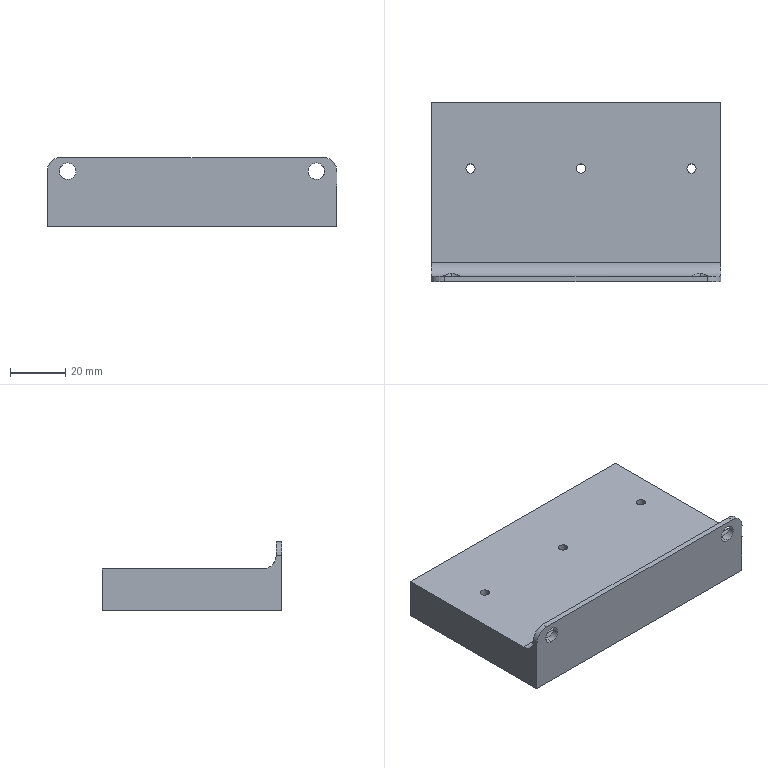Part | SolidWorks | features Fillet 2, Extrusion 1, HoleWzd 1, ICE 1 | 1 solid | 23 faces | box 105 x 65 x 24.968 mm | volume 104629 mm3 | cylinder 13 | plane 10 | commonest cylinder face diameters 3.3 x6 6 x4 10 x3
STEP:
#1=CARTESIAN_POINT('',(43.468,41.,-4.981));
#2=VERTEX_POINT('',#1);
#3=CARTESIAN_POINT('',(40.168,41.,-4.981));
#4=VERTEX_POINT('',#3);
#5=CARTESIAN_POINT('',(41.818,41.,-4.981));
#6=DIRECTION('',(0.,0.,-1.));
#7=DIRECTION('',(-1.,0.,0.));
#8=AXIS2_PLACEMENT_3D('',#5,#6,#7);
#9=CIRCLE('',#8,1.65);
#10=EDGE_CURVE('',#2,#4,#9,.T.);
#11=ORIENTED_EDGE('',*,*,#10,.F.);
#12=CARTESIAN_POINT('',(43.468,41.,-20.));
#13=VERTEX_POINT('',#12);
#14=CARTESIAN_POINT('',(43.468,41.,-20.));
#15=DIRECTION('',(0.,0.,-1.));
#16=VECTOR('',#15,1000.);
#17=LINE('',#14,#16);
#18=EDGE_CURVE('',#2,#13,#17,.T.);
#19=ORIENTED_EDGE('',*,*,#18,.T.);
#20=CARTESIAN_POINT('',(40.168,41.,-20.));
#21=VERTEX_POINT('',#20);
#22=CARTESIAN_POINT('',(41.818,41.,-20.));
#23=DIRECTION('',(0.,0.,-1.));
#24=DIRECTION('',(-1.,0.,0.));
#25=AXIS2_PLACEMENT_3D('',#22,#23,#24);
#26=CIRCLE('',#25,1.65);
#27=EDGE_CURVE('',#13,#21,#26,.T.);
#28=ORIENTED_EDGE('',*,*,#27,.T.);
#29=CARTESIAN_POINT('',(40.168,41.,-20.));
#30=DIRECTION('',(0.,0.,-1.));
#31=VECTOR('',#30,1000.);
#32=LINE('',#29,#31);
#33=EDGE_CURVE('',#4,#21,#32,.T.);
#34=ORIENTED_EDGE('',*,*,#33,.F.);
#35=EDGE_LOOP('',(#11,#19,#28,#34));
#36=FACE_OUTER_BOUND('',#35,.T.);
#37=CARTESIAN_POINT('',(41.818,41.,-20.));
#38=DIRECTION('',(0.,0.,-1.));
#39=DIRECTION('',(-1.,0.,0.));
#40=AXIS2_PLACEMENT_3D('',#37,#38,#39);
#41=CYLINDRICAL_SURFACE('',#40,1.65);
#42=ADVANCED_FACE('',(#36),#41,.F.);
#43=CARTESIAN_POINT('',(3.468,41.,-4.981));
#44=VERTEX_POINT('',#43);
#45=CARTESIAN_POINT('',(0.1683,41.,-4.981));
#46=VERTEX_POINT('',#45);
#47=CARTESIAN_POINT('',(1.818,41.,-4.981));
#48=DIRECTION('',(0.,0.,-1.));
#49=DIRECTION('',(-1.,0.,0.));
#50=AXIS2_PLACEMENT_3D('',#47,#48,#49);
#51=CIRCLE('',#50,1.65);
#52=EDGE_CURVE('',#44,#46,#51,.T.);
#53=ORIENTED_EDGE('',*,*,#52,.F.);
#54=CARTESIAN_POINT('',(3.468,41.,-20.));
#55=VERTEX_POINT('',#54);
#56=CARTESIAN_POINT('',(3.468,41.,-20.));
#57=DIRECTION('',(0.,0.,-1.));
#58=VECTOR('',#57,1000.);
#59=LINE('',#56,#58);
#60=EDGE_CURVE('',#44,#55,#59,.T.);
#61=ORIENTED_EDGE('',*,*,#60,.T.);
#62=CARTESIAN_POINT('',(0.1683,41.,-20.));
#63=VERTEX_POINT('',#62);
#64=CARTESIAN_POINT('',(1.818,41.,-20.));
#65=DIRECTION('',(0.,0.,-1.));
#66=DIRECTION('',(-1.,0.,0.));
#67=AXIS2_PLACEMENT_3D('',#64,#65,#66);
#68=CIRCLE('',#67,1.65);
#69=EDGE_CURVE('',#55,#63,#68,.T.);
#70=ORIENTED_EDGE('',*,*,#69,.T.);
#71=CARTESIAN_POINT('',(0.1683,41.,-20.));
#72=DIRECTION('',(0.,0.,-1.));
#73=VECTOR('',#72,1000.);
#74=LINE('',#71,#73);
#75=EDGE_CURVE('',#46,#63,#74,.T.);
#76=ORIENTED_EDGE('',*,*,#75,.F.);
#77=EDGE_LOOP('',(#53,#61,#70,#76));
#78=FACE_OUTER_BOUND('',#77,.T.);
#79=CARTESIAN_POINT('',(1.818,41.,-20.));
#80=DIRECTION('',(0.,0.,-1.));
#81=DIRECTION('',(-1.,0.,0.));
#82=AXIS2_PLACEMENT_3D('',#79,#80,#81);
#83=CYLINDRICAL_SURFACE('',#82,1.65);
#84=ADVANCED_FACE('',(#78),#83,.F.);
#85=CARTESIAN_POINT('',(-36.532,41.,-4.981));
#86=VERTEX_POINT('',#85);
#87=CARTESIAN_POINT('',(-39.832,41.,-4.981));
#88=VERTEX_POINT('',#87);
#89=CARTESIAN_POINT('',(-38.182,41.,-4.981));
#90=DIRECTION('',(0.,0.,-1.));
#91=DIRECTION('',(-1.,0.,0.));
#92=AXIS2_PLACEMENT_3D('',#89,#90,#91);
#93=CIRCLE('',#92,1.65);
#94=EDGE_CURVE('',#86,#88,#93,.T.);
#95=ORIENTED_EDGE('',*,*,#94,.F.);
#96=CARTESIAN_POINT('',(-36.532,41.,-20.));
#97=VERTEX_POINT('',#96);
#98=CARTESIAN_POINT('',(-36.532,41.,-20.));
#99=DIRECTION('',(0.,0.,-1.));
#100=VECTOR('',#99,1000.);
#101=LINE('',#98,#100);
#102=EDGE_CURVE('',#86,#97,#101,.T.);
#103=ORIENTED_EDGE('',*,*,#102,.T.);
#104=CARTESIAN_POINT('',(-39.832,41.,-20.));
#105=VERTEX_POINT('',#104);
#106=CARTESIAN_POINT('',(-38.182,41.,-20.));
#107=DIRECTION('',(0.,0.,-1.));
#108=DIRECTION('',(-1.,0.,0.));
#109=AXIS2_PLACEMENT_3D('',#106,#107,#108);
#110=CIRCLE('',#109,1.65);
#111=EDGE_CURVE('',#97,#105,#110,.T.);
#112=ORIENTED_EDGE('',*,*,#111,.T.);
#113=CARTESIAN_POINT('',(-39.832,41.,-20.));
#114=DIRECTION('',(0.,0.,-1.));
#115=VECTOR('',#114,1000.);
#116=LINE('',#113,#115);
#117=EDGE_CURVE('',#88,#105,#116,.T.);
#118=ORIENTED_EDGE('',*,*,#117,.F.);
#119=EDGE_LOOP('',(#95,#103,#112,#118));
#120=FACE_OUTER_BOUND('',#119,.T.);
#121=CARTESIAN_POINT('',(-38.182,41.,-20.));
#122=DIRECTION('',(0.,0.,-1.));
#123=DIRECTION('',(-1.,0.,0.));
#124=AXIS2_PLACEMENT_3D('',#121,#122,#123);
#125=CYLINDRICAL_SURFACE('',#124,1.65);
#126=ADVANCED_FACE('',(#120),#125,.F.);
#127=CARTESIAN_POINT('',(42.,2.,0.01879));
#128=VERTEX_POINT('',#127);
#129=CARTESIAN_POINT('',(45.,2.,3.));
#130=VERTEX_POINT('',#129);
#131=CARTESIAN_POINT('',(45.,2.,0.));
#132=DIRECTION('',(0.,1.,0.));
#133=DIRECTION('',(0.,0.,1.));
#134=AXIS2_PLACEMENT_3D('',#131,#132,#133);
#135=CIRCLE('',#134,3.);
#136=EDGE_CURVE('',#128,#130,#135,.T.);
#137=ORIENTED_EDGE('',*,*,#136,.T.);
#138=CARTESIAN_POINT('',(45.,0.,3.));
#139=VERTEX_POINT('',#138);
#140=CARTESIAN_POINT('',(45.,2.,3.));
#141=DIRECTION('',(0.,-1.,0.));
#142=VECTOR('',#141,1000.);
#143=LINE('',#140,#142);
#144=EDGE_CURVE('',#130,#139,#143,.T.);
#145=ORIENTED_EDGE('',*,*,#144,.T.);
#146=CARTESIAN_POINT('',(45.,0.,-3.));
#147=VERTEX_POINT('',#146);
#148=CARTESIAN_POINT('',(45.,0.,0.));
#149=DIRECTION('',(0.,1.,0.));
#150=DIRECTION('',(0.,0.,1.));
#151=AXIS2_PLACEMENT_3D('',#148,#149,#150);
#152=CIRCLE('',#151,3.);
#153=EDGE_CURVE('',#147,#139,#152,.T.);
#154=ORIENTED_EDGE('',*,*,#153,.F.);
#155=CARTESIAN_POINT('',(45.,3.014,-3.));
#156=VERTEX_POINT('',#155);
#157=CARTESIAN_POINT('',(45.,2.,-3.));
#158=DIRECTION('',(0.,-1.,0.));
#159=VECTOR('',#158,1000.);
#160=LINE('',#157,#159);
#161=EDGE_CURVE('',#156,#147,#160,.T.);
#162=ORIENTED_EDGE('',*,*,#161,.F.);
#163=CARTESIAN_POINT('',(45.,3.014,-3.));
#164=CARTESIAN_POINT('',(44.796,3.014,-3.));
#165=CARTESIAN_POINT('',(44.596,2.998,-2.979));
#166=CARTESIAN_POINT('',(44.203,2.939,-2.899));
#167=CARTESIAN_POINT('',(44.011,2.896,-2.839));
#168=CARTESIAN_POINT('',(43.65,2.794,-2.686));
#169=CARTESIAN_POINT('',(43.478,2.734,-2.592));
#170=CARTESIAN_POINT('',(43.158,2.609,-2.376));
#171=CARTESIAN_POINT('',(43.011,2.544,-2.254));
#172=CARTESIAN_POINT('',(42.739,2.415,-1.981));
#173=CARTESIAN_POINT('',(42.615,2.351,-1.831));
#174=CARTESIAN_POINT('',(42.401,2.236,-1.51));
#175=CARTESIAN_POINT('',(42.308,2.184,-1.339));
#176=CARTESIAN_POINT('',(42.155,2.095,-0.971));
#177=CARTESIAN_POINT('',(42.096,2.06,-0.7802));
#178=CARTESIAN_POINT('',(42.019,2.013,-0.3889));
#179=CARTESIAN_POINT('',(41.999,2.,-0.1861));
#180=CARTESIAN_POINT('',(42.,2.,0.01879));
#181=B_SPLINE_CURVE_WITH_KNOTS('',3,(#163,#164,#165,#166,#167,#168,#169,#170,#171,#172,#173,#174,#175,#176,#177,#178,#179,#180),.UNSPECIFIED.,.F.,.F.,(4,2,2,2,2,2,2,2,4),(0.004835,0.005439,0.006043,0.006647,0.007251,0.007855,0.008459,0.009064,0.009668),.UNSPECIFIED.);
#182=EDGE_CURVE('',#156,#128,#181,.T.);
#183=ORIENTED_EDGE('',*,*,#182,.T.);
#184=EDGE_LOOP('',(#137,#145,#154,#162,#183));
#185=FACE_OUTER_BOUND('',#184,.T.);
#186=CARTESIAN_POINT('',(45.,2.,0.));
#187=DIRECTION('',(0.,-1.,0.));
#188=DIRECTION('',(0.,0.,-1.));
#189=AXIS2_PLACEMENT_3D('',#186,#187,#188);
#190=CYLINDRICAL_SURFACE('',#189,3.);
#191=ADVANCED_FACE('',(#185),#190,.F.);
#192=CARTESIAN_POINT('',(-48.,2.,0.01879));
#193=VERTEX_POINT('',#192);
#194=CARTESIAN_POINT('',(-45.,2.,3.));
#195=VERTEX_POINT('',#194);
#196=CARTESIAN_POINT('',(-45.,2.,0.));
#197=DIRECTION('',(0.,1.,0.));
#198=DIRECTION('',(0.,0.,1.));
#199=AXIS2_PLACEMENT_3D('',#196,#197,#198);
#200=CIRCLE('',#199,3.);
#201=EDGE_CURVE('',#193,#195,#200,.T.);
#202=ORIENTED_EDGE('',*,*,#201,.T.);
#203=CARTESIAN_POINT('',(-45.,0.,3.));
#204=VERTEX_POINT('',#203);
#205=CARTESIAN_POINT('',(-45.,2.,3.));
#206=DIRECTION('',(0.,-1.,0.));
#207=VECTOR('',#206,1000.);
#208=LINE('',#205,#207);
#209=EDGE_CURVE('',#195,#204,#208,.T.);
#210=ORIENTED_EDGE('',*,*,#209,.T.);
#211=CARTESIAN_POINT('',(-45.,0.,-3.));
#212=VERTEX_POINT('',#211);
#213=CARTESIAN_POINT('',(-45.,0.,0.));
#214=DIRECTION('',(0.,1.,0.));
#215=DIRECTION('',(0.,0.,1.));
#216=AXIS2_PLACEMENT_3D('',#213,#214,#215);
#217=CIRCLE('',#216,3.);
#218=EDGE_CURVE('',#212,#204,#217,.T.);
#219=ORIENTED_EDGE('',*,*,#218,.F.);
#220=CARTESIAN_POINT('',(-45.,3.014,-3.));
#221=VERTEX_POINT('',#220);
#222=CARTESIAN_POINT('',(-45.,2.,-3.));
#223=DIRECTION('',(0.,-1.,0.));
#224=VECTOR('',#223,1000.);
#225=LINE('',#222,#224);
#226=EDGE_CURVE('',#221,#212,#225,.T.);
#227=ORIENTED_EDGE('',*,*,#226,.F.);
#228=CARTESIAN_POINT('',(-45.,3.014,-3.));
#229=CARTESIAN_POINT('',(-45.204,3.014,-3.));
#230=CARTESIAN_POINT('',(-45.404,2.998,-2.979));
#231=CARTESIAN_POINT('',(-45.797,2.939,-2.899));
#232=CARTESIAN_POINT('',(-45.989,2.896,-2.839));
#233=CARTESIAN_POINT('',(-46.35,2.794,-2.686));
#234=CARTESIAN_POINT('',(-46.522,2.734,-2.592));
#235=CARTESIAN_POINT('',(-46.842,2.609,-2.376));
#236=CARTESIAN_POINT('',(-46.989,2.544,-2.254));
#237=CARTESIAN_POINT('',(-47.261,2.415,-1.981));
#238=CARTESIAN_POINT('',(-47.385,2.351,-1.831));
#239=CARTESIAN_POINT('',(-47.599,2.236,-1.51));
#240=CARTESIAN_POINT('',(-47.692,2.184,-1.339));
#241=CARTESIAN_POINT('',(-47.845,2.095,-0.971));
#242=CARTESIAN_POINT('',(-47.904,2.06,-0.7802));
#243=CARTESIAN_POINT('',(-47.981,2.013,-0.3889));
#244=CARTESIAN_POINT('',(-48.001,2.,-0.1861));
#245=CARTESIAN_POINT('',(-48.,2.,0.01879));
#246=B_SPLINE_CURVE_WITH_KNOTS('',3,(#228,#229,#230,#231,#232,#233,#234,#235,#236,#237,#238,#239,#240,#241,#242,#243,#244,#245),.UNSPECIFIED.,.F.,.F.,(4,2,2,2,2,2,2,2,4),(0.004835,0.005439,0.006043,0.006647,0.007251,0.007855,0.008459,0.009064,0.009668),.UNSPECIFIED.);
#247=EDGE_CURVE('',#221,#193,#246,.T.);
#248=ORIENTED_EDGE('',*,*,#247,.T.);
#249=EDGE_LOOP('',(#202,#210,#219,#227,#248));
#250=FACE_OUTER_BOUND('',#249,.T.);
#251=CARTESIAN_POINT('',(-45.,2.,0.));
#252=DIRECTION('',(0.,-1.,0.));
#253=DIRECTION('',(0.,0.,-1.));
#254=AXIS2_PLACEMENT_3D('',#251,#252,#253);
#255=CYLINDRICAL_SURFACE('',#254,3.);
#256=ADVANCED_FACE('',(#250),#255,.F.);
#257=CARTESIAN_POINT('',(41.818,41.,-4.981));
#258=DIRECTION('',(0.,0.,-1.));
#259=DIRECTION('',(-1.,0.,0.));
#260=AXIS2_PLACEMENT_3D('',#257,#258,#259);
#261=CIRCLE('',#260,1.65);
#262=EDGE_CURVE('',#4,#2,#261,.T.);
#263=ORIENTED_EDGE('',*,*,#262,.T.);
#264=ORIENTED_EDGE('',*,*,#10,.T.);
#265=EDGE_LOOP('',(#263,#264));
#266=FACE_BOUND('',#265,.T.);
#267=CARTESIAN_POINT('',(1.818,41.,-4.981));
#268=DIRECTION('',(0.,0.,-1.));
#269=DIRECTION('',(-1.,0.,0.));
#270=AXIS2_PLACEMENT_3D('',#267,#268,#269);
#271=CIRCLE('',#270,1.65);
#272=EDGE_CURVE('',#46,#44,#271,.T.);
#273=ORIENTED_EDGE('',*,*,#272,.T.);
#274=ORIENTED_EDGE('',*,*,#52,.T.);
#275=EDGE_LOOP('',(#273,#274));
#276=FACE_BOUND('',#275,.T.);
#277=CARTESIAN_POINT('',(-38.182,41.,-4.981));
#278=DIRECTION('',(0.,0.,-1.));
#279=DIRECTION('',(-1.,0.,0.));
#280=AXIS2_PLACEMENT_3D('',#277,#278,#279);
#281=CIRCLE('',#280,1.65);
#282=EDGE_CURVE('',#88,#86,#281,.T.);
#283=ORIENTED_EDGE('',*,*,#282,.T.);
#284=ORIENTED_EDGE('',*,*,#94,.T.);
#285=EDGE_LOOP('',(#283,#284));
#286=FACE_BOUND('',#285,.T.);
#287=CARTESIAN_POINT('',(-52.5,65.,-4.981));
#288=VERTEX_POINT('',#287);
#289=CARTESIAN_POINT('',(-52.5,7.,-4.981));
#290=VERTEX_POINT('',#289);
#291=CARTESIAN_POINT('',(-52.5,65.,-4.981));
#292=DIRECTION('',(0.,-1.,0.));
#293=VECTOR('',#292,1000.);
#294=LINE('',#291,#293);
#295=EDGE_CURVE('',#288,#290,#294,.T.);
#296=ORIENTED_EDGE('',*,*,#295,.T.);
#297=CARTESIAN_POINT('',(52.5,7.,-4.981));
#298=VERTEX_POINT('',#297);
#299=CARTESIAN_POINT('',(0.,7.,-4.981));
#300=DIRECTION('',(1.,0.,0.));
#301=VECTOR('',#300,1000.);
#302=LINE('',#299,#301);
#303=EDGE_CURVE('',#290,#298,#302,.T.);
#304=ORIENTED_EDGE('',*,*,#303,.T.);
#305=CARTESIAN_POINT('',(52.5,65.,-4.981));
#306=VERTEX_POINT('',#305);
#307=CARTESIAN_POINT('',(52.5,65.,-4.981));
#308=DIRECTION('',(0.,-1.,0.));
#309=VECTOR('',#308,1000.);
#310=LINE('',#307,#309);
#311=EDGE_CURVE('',#306,#298,#310,.T.);
#312=ORIENTED_EDGE('',*,*,#311,.F.);
#313=CARTESIAN_POINT('',(0.,65.,-4.981));
#314=DIRECTION('',(1.,0.,0.));
#315=VECTOR('',#314,1000.);
#316=LINE('',#313,#315);
#317=EDGE_CURVE('',#288,#306,#316,.T.);
#318=ORIENTED_EDGE('',*,*,#317,.F.);
#319=EDGE_LOOP('',(#296,#304,#312,#318));
#320=FACE_OUTER_BOUND('',#319,.T.);
#321=CARTESIAN_POINT('',(0.,65.,-4.981));
#322=DIRECTION('',(0.,0.,-1.));
#323=DIRECTION('',(-1.,0.,0.));
#324=AXIS2_PLACEMENT_3D('',#321,#322,#323);
#325=PLANE('',#324);
#326=ADVANCED_FACE('',(#266,#276,#286,#320),#325,.F.);
#327=CARTESIAN_POINT('',(52.5,0.,-4.981));
#328=VERTEX_POINT('',#327);
#329=CARTESIAN_POINT('',(52.5,0.,-20.));
#330=VERTEX_POINT('',#329);
#331=CARTESIAN_POINT('',(52.5,0.,0.));
#332=DIRECTION('',(0.,0.,-1.));
#333=VECTOR('',#332,1000.);
#334=LINE('',#331,#333);
#335=EDGE_CURVE('',#328,#330,#334,.T.);
#336=ORIENTED_EDGE('',*,*,#335,.T.);
#337=CARTESIAN_POINT('',(52.5,65.,-20.));
#338=VERTEX_POINT('',#337);
#339=CARTESIAN_POINT('',(52.5,65.,-20.));
#340=DIRECTION('',(0.,-1.,0.));
#341=VECTOR('',#340,1000.);
#342=LINE('',#339,#341);
#343=EDGE_CURVE('',#338,#330,#342,.T.);
#344=ORIENTED_EDGE('',*,*,#343,.F.);
#345=CARTESIAN_POINT('',(52.5,65.,0.));
#346=DIRECTION('',(0.,0.,-1.));
#347=VECTOR('',#346,1000.);
#348=LINE('',#345,#347);
#349=EDGE_CURVE('',#306,#338,#348,.T.);
#350=ORIENTED_EDGE('',*,*,#349,.F.);
#351=ORIENTED_EDGE('',*,*,#311,.T.);
#352=CARTESIAN_POINT('',(52.5,65.,-4.981));
#353=DIRECTION('',(0.,-1.,0.));
#354=VECTOR('',#353,1000.);
#355=LINE('',#352,#354);
#356=EDGE_CURVE('',#298,#328,#355,.T.);
#357=ORIENTED_EDGE('',*,*,#356,.T.);
#358=EDGE_LOOP('',(#336,#344,#350,#351,#357));
#359=FACE_OUTER_BOUND('',#358,.T.);
#360=CARTESIAN_POINT('',(52.5,65.,0.));
#361=DIRECTION('',(-1.,0.,0.));
#362=DIRECTION('',(0.,0.,1.));
#363=AXIS2_PLACEMENT_3D('',#360,#361,#362);
#364=PLANE('',#363);
#365=ADVANCED_FACE('',(#359),#364,.F.);
#366=CARTESIAN_POINT('',(41.818,41.,-20.));
#367=DIRECTION('',(0.,0.,-1.));
#368=DIRECTION('',(-1.,0.,0.));
#369=AXIS2_PLACEMENT_3D('',#366,#367,#368);
#370=CIRCLE('',#369,1.65);
#371=EDGE_CURVE('',#21,#13,#370,.T.);
#372=ORIENTED_EDGE('',*,*,#371,.F.);
#373=ORIENTED_EDGE('',*,*,#27,.F.);
#374=EDGE_LOOP('',(#372,#373));
#375=FACE_BOUND('',#374,.T.);
#376=CARTESIAN_POINT('',(1.818,41.,-20.));
#377=DIRECTION('',(0.,0.,-1.));
#378=DIRECTION('',(-1.,0.,0.));
#379=AXIS2_PLACEMENT_3D('',#376,#377,#378);
#380=CIRCLE('',#379,1.65);
#381=EDGE_CURVE('',#63,#55,#380,.T.);
#382=ORIENTED_EDGE('',*,*,#381,.F.);
#383=ORIENTED_EDGE('',*,*,#69,.F.);
#384=EDGE_LOOP('',(#382,#383));
#385=FACE_BOUND('',#384,.T.);
#386=CARTESIAN_POINT('',(-38.182,41.,-20.));
#387=DIRECTION('',(0.,0.,-1.));
#388=DIRECTION('',(-1.,0.,0.));
#389=AXIS2_PLACEMENT_3D('',#386,#387,#388);
#390=CIRCLE('',#389,1.65);
#391=EDGE_CURVE('',#105,#97,#390,.T.);
#392=ORIENTED_EDGE('',*,*,#391,.F.);
#393=ORIENTED_EDGE('',*,*,#111,.F.);
#394=EDGE_LOOP('',(#392,#393));
#395=FACE_BOUND('',#394,.T.);
#396=CARTESIAN_POINT('',(-52.5,0.,-20.));
#397=VERTEX_POINT('',#396);
#398=CARTESIAN_POINT('',(0.,0.,-20.));
#399=DIRECTION('',(1.,0.,0.));
#400=VECTOR('',#399,1000.);
#401=LINE('',#398,#400);
#402=EDGE_CURVE('',#397,#330,#401,.T.);
#403=ORIENTED_EDGE('',*,*,#402,.F.);
#404=CARTESIAN_POINT('',(-52.5,65.,-20.));
#405=VERTEX_POINT('',#404);
#406=CARTESIAN_POINT('',(-52.5,65.,-20.));
#407=DIRECTION('',(0.,-1.,0.));
#408=VECTOR('',#407,1000.);
#409=LINE('',#406,#408);
#410=EDGE_CURVE('',#405,#397,#409,.T.);
#411=ORIENTED_EDGE('',*,*,#410,.F.);
#412=CARTESIAN_POINT('',(0.,65.,-20.));
#413=DIRECTION('',(1.,0.,0.));
#414=VECTOR('',#413,1000.);
#415=LINE('',#412,#414);
#416=EDGE_CURVE('',#405,#338,#415,.T.);
#417=ORIENTED_EDGE('',*,*,#416,.T.);
#418=ORIENTED_EDGE('',*,*,#343,.T.);
#419=EDGE_LOOP('',(#403,#411,#417,#418));
#420=FACE_OUTER_BOUND('',#419,.T.);
#421=CARTESIAN_POINT('',(0.,65.,-20.));
#422=DIRECTION('',(0.,0.,-1.));
#423=DIRECTION('',(-1.,0.,0.));
#424=AXIS2_PLACEMENT_3D('',#421,#422,#423);
#425=PLANE('',#424);
#426=ADVANCED_FACE('',(#375,#385,#395,#420),#425,.T.);
#427=CARTESIAN_POINT('',(-52.5,0.,-0.0316));
#428=VERTEX_POINT('',#427);
#429=CARTESIAN_POINT('',(-52.5,0.,0.));
#430=DIRECTION('',(0.,0.,-1.));
#431=VECTOR('',#430,1000.);
#432=LINE('',#429,#431);
#433=EDGE_CURVE('',#428,#397,#432,.T.);
#434=ORIENTED_EDGE('',*,*,#433,.F.);
#435=CARTESIAN_POINT('',(-52.5,2.,-0.0316));
#436=VERTEX_POINT('',#435);
#437=CARTESIAN_POINT('',(-52.5,2.,-0.0316));
#438=DIRECTION('',(0.,1.,0.));
#439=VECTOR('',#438,1000.);
#440=LINE('',#437,#439);
#441=EDGE_CURVE('',#428,#436,#440,.T.);
#442=ORIENTED_EDGE('',*,*,#441,.T.);
#443=CARTESIAN_POINT('',(-52.5,7.,0.01879));
#444=DIRECTION('',(1.,0.,0.));
#445=DIRECTION('',(0.,0.,1.));
#446=AXIS2_PLACEMENT_3D('',#443,#444,#445);
#447=CIRCLE('',#446,5.);
#448=EDGE_CURVE('',#436,#290,#447,.T.);
#449=ORIENTED_EDGE('',*,*,#448,.T.);
#450=ORIENTED_EDGE('',*,*,#295,.F.);
#451=CARTESIAN_POINT('',(-52.5,65.,0.));
#452=DIRECTION('',(0.,0.,-1.));
#453=VECTOR('',#452,1000.);
#454=LINE('',#451,#453);
#455=EDGE_CURVE('',#288,#405,#454,.T.);
#456=ORIENTED_EDGE('',*,*,#455,.T.);
#457=ORIENTED_EDGE('',*,*,#410,.T.);
#458=EDGE_LOOP('',(#434,#442,#449,#450,#456,#457));
#459=FACE_OUTER_BOUND('',#458,.T.);
#460=CARTESIAN_POINT('',(-52.5,65.,0.));
#461=DIRECTION('',(-1.,0.,0.));
#462=DIRECTION('',(0.,0.,1.));
#463=AXIS2_PLACEMENT_3D('',#460,#461,#462);
#464=PLANE('',#463);
#465=ADVANCED_FACE('',(#459),#464,.T.);
#466=ORIENTED_EDGE('',*,*,#317,.T.);
#467=ORIENTED_EDGE('',*,*,#349,.T.);
#468=ORIENTED_EDGE('',*,*,#416,.F.);
#469=ORIENTED_EDGE('',*,*,#455,.F.);
#470=EDGE_LOOP('',(#466,#467,#468,#469));
#471=FACE_OUTER_BOUND('',#470,.T.);
#472=CARTESIAN_POINT('',(0.,65.,0.));
#473=DIRECTION('',(0.,1.,0.));
#474=DIRECTION('',(0.,0.,1.));
#475=AXIS2_PLACEMENT_3D('',#472,#473,#474);
#476=PLANE('',#475);
#477=ADVANCED_FACE('',(#471),#476,.T.);
#478=CARTESIAN_POINT('',(52.5,0.,-0.0316));
#479=VERTEX_POINT('',#478);
#480=CARTESIAN_POINT('',(52.5,0.,-4.981));
#481=VERTEX_POINT('',#480);
#482=CARTESIAN_POINT('',(52.5,0.,-4.981));
#483=DIRECTION('',(0.,0.,-1.));
#484=VECTOR('',#483,1000.);
#485=LINE('',#482,#484);
#486=EDGE_CURVE('',#479,#481,#485,.T.);
#487=ORIENTED_EDGE('',*,*,#486,.F.);
#488=CARTESIAN_POINT('',(47.5,0.,4.968));
#489=VERTEX_POINT('',#488);
#490=CARTESIAN_POINT('',(47.5,0.,-0.0316));
#491=DIRECTION('',(0.,-1.,0.));
#492=DIRECTION('',(0.,0.,1.));
#493=AXIS2_PLACEMENT_3D('',#490,#491,#492);
#494=CIRCLE('',#493,5.);
#495=EDGE_CURVE('',#479,#489,#494,.T.);
#496=ORIENTED_EDGE('',*,*,#495,.T.);
#497=CARTESIAN_POINT('',(-47.5,0.,4.968));
#498=VERTEX_POINT('',#497);
#499=CARTESIAN_POINT('',(-52.5,0.,4.968));
#500=DIRECTION('',(1.,0.,0.));
#501=VECTOR('',#500,1000.);
#502=LINE('',#499,#501);
#503=EDGE_CURVE('',#498,#489,#502,.T.);
#504=ORIENTED_EDGE('',*,*,#503,.F.);
#505=CARTESIAN_POINT('',(-47.5,0.,-0.0316));
#506=DIRECTION('',(0.,-1.,0.));
#507=DIRECTION('',(0.,0.,1.));
#508=AXIS2_PLACEMENT_3D('',#505,#506,#507);
#509=CIRCLE('',#508,5.);
#510=EDGE_CURVE('',#498,#428,#509,.T.);
#511=ORIENTED_EDGE('',*,*,#510,.T.);
#512=ORIENTED_EDGE('',*,*,#433,.T.);
#513=ORIENTED_EDGE('',*,*,#402,.T.);
#514=ORIENTED_EDGE('',*,*,#335,.F.);
#515=CARTESIAN_POINT('',(-52.5,0.,-4.981));
#516=DIRECTION('',(-1.,0.,0.));
#517=VECTOR('',#516,1000.);
#518=LINE('',#515,#517);
#519=EDGE_CURVE('',#481,#328,#518,.T.);
#520=ORIENTED_EDGE('',*,*,#519,.F.);
#521=EDGE_LOOP('',(#487,#496,#504,#511,#512,#513,#514,#520));
#522=FACE_OUTER_BOUND('',#521,.T.);
#523=ORIENTED_EDGE('',*,*,#218,.T.);
#524=CARTESIAN_POINT('',(-45.,0.,0.));
#525=DIRECTION('',(0.,1.,0.));
#526=DIRECTION('',(0.,0.,1.));
#527=AXIS2_PLACEMENT_3D('',#524,#525,#526);
#528=CIRCLE('',#527,3.);
#529=EDGE_CURVE('',#204,#212,#528,.T.);
#530=ORIENTED_EDGE('',*,*,#529,.T.);
#531=EDGE_LOOP('',(#523,#530));
#532=FACE_BOUND('',#531,.T.);
#533=ORIENTED_EDGE('',*,*,#153,.T.);
#534=CARTESIAN_POINT('',(45.,0.,0.));
#535=DIRECTION('',(0.,1.,0.));
#536=DIRECTION('',(0.,0.,1.));
#537=AXIS2_PLACEMENT_3D('',#534,#535,#536);
#538=CIRCLE('',#537,3.);
#539=EDGE_CURVE('',#139,#147,#538,.T.);
#540=ORIENTED_EDGE('',*,*,#539,.T.);
#541=EDGE_LOOP('',(#533,#540));
#542=FACE_BOUND('',#541,.T.);
#543=CARTESIAN_POINT('',(0.,0.,0.));
#544=DIRECTION('',(0.,1.,0.));
#545=DIRECTION('',(0.,0.,1.));
#546=AXIS2_PLACEMENT_3D('',#543,#544,#545);
#547=PLANE('',#546);
#548=ADVANCED_FACE('',(#522,#532,#542),#547,.F.);
#549=CARTESIAN_POINT('',(47.5,2.,4.968));
#550=VERTEX_POINT('',#549);
#551=CARTESIAN_POINT('',(52.5,2.,0.01879));
#552=VERTEX_POINT('',#551);
#553=CARTESIAN_POINT('',(47.5,2.,-0.0316));
#554=DIRECTION('',(0.,1.,0.));
#555=DIRECTION('',(0.,0.,1.));
#556=AXIS2_PLACEMENT_3D('',#553,#554,#555);
#557=CIRCLE('',#556,5.);
#558=EDGE_CURVE('',#550,#552,#557,.T.);
#559=ORIENTED_EDGE('',*,*,#558,.T.);
#560=CARTESIAN_POINT('',(48.,2.,0.01879));
#561=VERTEX_POINT('',#560);
#562=CARTESIAN_POINT('',(0.,2.,0.01879));
#563=DIRECTION('',(-1.,0.,0.));
#564=VECTOR('',#563,1000.);
#565=LINE('',#562,#564);
#566=EDGE_CURVE('',#552,#561,#565,.T.);
#567=ORIENTED_EDGE('',*,*,#566,.T.);
#568=CARTESIAN_POINT('',(45.,2.,0.));
#569=DIRECTION('',(0.,1.,0.));
#570=DIRECTION('',(0.,0.,1.));
#571=AXIS2_PLACEMENT_3D('',#568,#569,#570);
#572=CIRCLE('',#571,3.);
#573=EDGE_CURVE('',#130,#561,#572,.T.);
#574=ORIENTED_EDGE('',*,*,#573,.F.);
#575=ORIENTED_EDGE('',*,*,#136,.F.);
#576=CARTESIAN_POINT('',(-42.,2.,0.01879));
#577=VERTEX_POINT('',#576);
#578=CARTESIAN_POINT('',(0.,2.,0.01879));
#579=DIRECTION('',(-1.,0.,0.));
#580=VECTOR('',#579,1000.);
#581=LINE('',#578,#580);
#582=EDGE_CURVE('',#128,#577,#581,.T.);
#583=ORIENTED_EDGE('',*,*,#582,.T.);
#584=CARTESIAN_POINT('',(-45.,2.,0.));
#585=DIRECTION('',(0.,1.,0.));
#586=DIRECTION('',(0.,0.,1.));
#587=AXIS2_PLACEMENT_3D('',#584,#585,#586);
#588=CIRCLE('',#587,3.);
#589=EDGE_CURVE('',#195,#577,#588,.T.);
#590=ORIENTED_EDGE('',*,*,#589,.F.);
#591=ORIENTED_EDGE('',*,*,#201,.F.);
#592=CARTESIAN_POINT('',(-52.5,2.,0.01879));
#593=VERTEX_POINT('',#592);
#594=CARTESIAN_POINT('',(0.,2.,0.01879));
#595=DIRECTION('',(-1.,0.,0.));
#596=VECTOR('',#595,1000.);
#597=LINE('',#594,#596);
#598=EDGE_CURVE('',#193,#593,#597,.T.);
#599=ORIENTED_EDGE('',*,*,#598,.T.);
#600=CARTESIAN_POINT('',(-47.5,2.,4.968));
#601=VERTEX_POINT('',#600);
#602=CARTESIAN_POINT('',(-47.5,2.,-0.0316));
#603=DIRECTION('',(0.,1.,0.));
#604=DIRECTION('',(0.,0.,1.));
#605=AXIS2_PLACEMENT_3D('',#602,#603,#604);
#606=CIRCLE('',#605,5.);
#607=EDGE_CURVE('',#593,#601,#606,.T.);
#608=ORIENTED_EDGE('',*,*,#607,.T.);
#609=CARTESIAN_POINT('',(-52.5,2.,4.968));
#610=DIRECTION('',(1.,0.,0.));
#611=VECTOR('',#610,1000.);
#612=LINE('',#609,#611);
#613=EDGE_CURVE('',#601,#550,#612,.T.);
#614=ORIENTED_EDGE('',*,*,#613,.T.);
#615=EDGE_LOOP('',(#559,#567,#574,#575,#583,#590,#591,#599,#608,#614));
#616=FACE_OUTER_BOUND('',#615,.T.);
#617=CARTESIAN_POINT('',(0.,2.,0.));
#618=DIRECTION('',(0.,1.,0.));
#619=DIRECTION('',(0.,0.,1.));
#620=AXIS2_PLACEMENT_3D('',#617,#618,#619);
#621=PLANE('',#620);
#622=ADVANCED_FACE('',(#616),#621,.T.);
#623=ORIENTED_EDGE('',*,*,#503,.T.);
#624=CARTESIAN_POINT('',(47.5,2.,4.968));
#625=DIRECTION('',(0.,1.,0.));
#626=VECTOR('',#625,1000.);
#627=LINE('',#624,#626);
#628=EDGE_CURVE('',#489,#550,#627,.T.);
#629=ORIENTED_EDGE('',*,*,#628,.T.);
#630=ORIENTED_EDGE('',*,*,#613,.F.);
#631=CARTESIAN_POINT('',(-47.5,0.,4.968));
#632=DIRECTION('',(0.,-1.,0.));
#633=VECTOR('',#632,1000.);
#634=LINE('',#631,#633);
#635=EDGE_CURVE('',#601,#498,#634,.T.);
#636=ORIENTED_EDGE('',*,*,#635,.T.);
#637=EDGE_LOOP('',(#623,#629,#630,#636));
#638=FACE_OUTER_BOUND('',#637,.T.);
#639=CARTESIAN_POINT('',(-52.5,2.,4.968));
#640=DIRECTION('',(0.,0.,-1.));
#641=DIRECTION('',(-1.,0.,0.));
#642=AXIS2_PLACEMENT_3D('',#639,#640,#641);
#643=PLANE('',#642);
#644=ADVANCED_FACE('',(#638),#643,.F.);
#645=CARTESIAN_POINT('',(52.5,7.,-4.981));
#646=VERTEX_POINT('',#645);
#647=CARTESIAN_POINT('',(52.5,2.,-4.981));
#648=DIRECTION('',(0.,-1.,0.));
#649=VECTOR('',#648,1000.);
#650=LINE('',#647,#649);
#651=EDGE_CURVE('',#646,#481,#650,.T.);
#652=ORIENTED_EDGE('',*,*,#651,.F.);
#653=CARTESIAN_POINT('',(52.5,2.,-0.0316));
#654=VERTEX_POINT('',#653);
#655=CARTESIAN_POINT('',(52.5,7.,0.01879));
#656=DIRECTION('',(-1.,0.,0.));
#657=DIRECTION('',(0.,0.,1.));
#658=AXIS2_PLACEMENT_3D('',#655,#656,#657);
#659=CIRCLE('',#658,5.);
#660=EDGE_CURVE('',#646,#654,#659,.T.);
#661=ORIENTED_EDGE('',*,*,#660,.T.);
#662=CARTESIAN_POINT('',(52.5,2.,-0.0316));
#663=DIRECTION('',(0.,-1.,0.));
#664=VECTOR('',#663,1000.);
#665=LINE('',#662,#664);
#666=EDGE_CURVE('',#654,#479,#665,.T.);
#667=ORIENTED_EDGE('',*,*,#666,.T.);
#668=ORIENTED_EDGE('',*,*,#486,.T.);
#669=EDGE_LOOP('',(#652,#661,#667,#668));
#670=FACE_OUTER_BOUND('',#669,.T.);
#671=CARTESIAN_POINT('',(52.5,2.,-4.981));
#672=DIRECTION('',(-1.,0.,0.));
#673=DIRECTION('',(0.,0.,1.));
#674=AXIS2_PLACEMENT_3D('',#671,#672,#673);
#675=PLANE('',#674);
#676=ADVANCED_FACE('',(#670),#675,.F.);
#677=ORIENTED_EDGE('',*,*,#356,.F.);
#678=CARTESIAN_POINT('',(52.5,7.,-4.981));
#679=DIRECTION('',(1.,0.,0.));
#680=VECTOR('',#679,1000.);
#681=LINE('',#678,#680);
#682=EDGE_CURVE('',#298,#646,#681,.T.);
#683=ORIENTED_EDGE('',*,*,#682,.T.);
#684=ORIENTED_EDGE('',*,*,#651,.T.);
#685=ORIENTED_EDGE('',*,*,#519,.T.);
#686=EDGE_LOOP('',(#677,#683,#684,#685));
#687=FACE_OUTER_BOUND('',#686,.T.);
#688=CARTESIAN_POINT('',(-52.5,2.,-4.981));
#689=DIRECTION('',(0.,0.,1.));
#690=DIRECTION('',(1.,0.,0.));
#691=AXIS2_PLACEMENT_3D('',#688,#689,#690);
#692=PLANE('',#691);
#693=ADVANCED_FACE('',(#687),#692,.F.);
#694=ORIENTED_EDGE('',*,*,#209,.F.);
#695=ORIENTED_EDGE('',*,*,#589,.T.);
#696=CARTESIAN_POINT('',(-42.,2.,0.01879));
#697=CARTESIAN_POINT('',(-41.999,2.,-0.1859));
#698=CARTESIAN_POINT('',(-42.018,2.013,-0.3863));
#699=CARTESIAN_POINT('',(-42.096,2.06,-0.7794));
#700=CARTESIAN_POINT('',(-42.156,2.096,-0.9737));
#701=CARTESIAN_POINT('',(-42.384,2.228,-1.52));
#702=CARTESIAN_POINT('',(-42.606,2.352,-1.848));
#703=CARTESIAN_POINT('',(-43.012,2.544,-2.255));
#704=CARTESIAN_POINT('',(-43.161,2.61,-2.378));
#705=CARTESIAN_POINT('',(-43.481,2.735,-2.594));
#706=CARTESIAN_POINT('',(-43.649,2.794,-2.686));
#707=CARTESIAN_POINT('',(-44.009,2.896,-2.838));
#708=CARTESIAN_POINT('',(-44.202,2.939,-2.899));
#709=CARTESIAN_POINT('',(-44.593,2.998,-2.979));
#710=CARTESIAN_POINT('',(-44.796,3.014,-3.));
#711=CARTESIAN_POINT('',(-45.,3.014,-3.));
#712=B_SPLINE_CURVE_WITH_KNOTS('',3,(#696,#697,#698,#699,#700,#701,#702,#703,#704,#705,#706,#707,#708,#709,#710,#711),.UNSPECIFIED.,.F.,.F.,(4,2,2,2,2,2,2,4),(0.,0.0006044,0.001209,0.002417,0.003022,0.003626,0.004231,0.004835),.UNSPECIFIED.);
#713=EDGE_CURVE('',#577,#221,#712,.T.);
#714=ORIENTED_EDGE('',*,*,#713,.T.);
#715=ORIENTED_EDGE('',*,*,#226,.T.);
#716=ORIENTED_EDGE('',*,*,#529,.F.);
#717=EDGE_LOOP('',(#694,#695,#714,#715,#716));
#718=FACE_OUTER_BOUND('',#717,.T.);
#719=CARTESIAN_POINT('',(-45.,2.,0.));
#720=DIRECTION('',(0.,-1.,0.));
#721=DIRECTION('',(0.,0.,-1.));
#722=AXIS2_PLACEMENT_3D('',#719,#720,#721);
#723=CYLINDRICAL_SURFACE('',#722,3.);
#724=ADVANCED_FACE('',(#718),#723,.F.);
#725=ORIENTED_EDGE('',*,*,#144,.F.);
#726=ORIENTED_EDGE('',*,*,#573,.T.);
#727=CARTESIAN_POINT('',(48.,2.,0.01879));
#728=CARTESIAN_POINT('',(48.001,2.,-0.1859));
#729=CARTESIAN_POINT('',(47.982,2.013,-0.3863));
#730=CARTESIAN_POINT('',(47.904,2.06,-0.7794));
#731=CARTESIAN_POINT('',(47.844,2.096,-0.9737));
#732=CARTESIAN_POINT('',(47.616,2.228,-1.52));
#733=CARTESIAN_POINT('',(47.394,2.352,-1.848));
#734=CARTESIAN_POINT('',(46.988,2.544,-2.255));
#735=CARTESIAN_POINT('',(46.839,2.61,-2.378));
#736=CARTESIAN_POINT('',(46.519,2.735,-2.594));
#737=CARTESIAN_POINT('',(46.351,2.794,-2.686));
#738=CARTESIAN_POINT('',(45.991,2.896,-2.838));
#739=CARTESIAN_POINT('',(45.798,2.939,-2.899));
#740=CARTESIAN_POINT('',(45.407,2.998,-2.979));
#741=CARTESIAN_POINT('',(45.204,3.014,-3.));
#742=CARTESIAN_POINT('',(45.,3.014,-3.));
#743=B_SPLINE_CURVE_WITH_KNOTS('',3,(#727,#728,#729,#730,#731,#732,#733,#734,#735,#736,#737,#738,#739,#740,#741,#742),.UNSPECIFIED.,.F.,.F.,(4,2,2,2,2,2,2,4),(0.,0.0006044,0.001209,0.002417,0.003022,0.003626,0.004231,0.004835),.UNSPECIFIED.);
#744=EDGE_CURVE('',#561,#156,#743,.T.);
#745=ORIENTED_EDGE('',*,*,#744,.T.);
#746=ORIENTED_EDGE('',*,*,#161,.T.);
#747=ORIENTED_EDGE('',*,*,#539,.F.);
#748=EDGE_LOOP('',(#725,#726,#745,#746,#747));
#749=FACE_OUTER_BOUND('',#748,.T.);
#750=CARTESIAN_POINT('',(45.,2.,0.));
#751=DIRECTION('',(0.,-1.,0.));
#752=DIRECTION('',(0.,0.,-1.));
#753=AXIS2_PLACEMENT_3D('',#750,#751,#752);
#754=CYLINDRICAL_SURFACE('',#753,3.);
#755=ADVANCED_FACE('',(#749),#754,.F.);
#756=ORIENTED_EDGE('',*,*,#558,.F.);
#757=ORIENTED_EDGE('',*,*,#628,.F.);
#758=ORIENTED_EDGE('',*,*,#495,.F.);
#759=ORIENTED_EDGE('',*,*,#666,.F.);
#760=CARTESIAN_POINT('',(52.5,2.,-0.0316));
#761=CARTESIAN_POINT('',(52.5,2.,-0.01481));
#762=CARTESIAN_POINT('',(52.5,2.,0.001991));
#763=CARTESIAN_POINT('',(52.5,2.,0.01879));
#764=B_SPLINE_CURVE_WITH_KNOTS('',3,(#760,#761,#762,#763),.UNSPECIFIED.,.F.,.F.,(4,4),(0.,0.00005039),.UNSPECIFIED.);
#765=EDGE_CURVE('',#654,#552,#764,.T.);
#766=ORIENTED_EDGE('',*,*,#765,.T.);
#767=EDGE_LOOP('',(#756,#757,#758,#759,#766));
#768=FACE_OUTER_BOUND('',#767,.T.);
#769=CARTESIAN_POINT('',(47.5,2.,-0.0316));
#770=DIRECTION('',(0.,-1.,0.));
#771=DIRECTION('',(0.,0.,-1.));
#772=AXIS2_PLACEMENT_3D('',#769,#770,#771);
#773=CYLINDRICAL_SURFACE('',#772,5.);
#774=ADVANCED_FACE('',(#768),#773,.T.);
#775=ORIENTED_EDGE('',*,*,#607,.F.);
#776=CARTESIAN_POINT('',(-52.5,2.,0.01879));
#777=CARTESIAN_POINT('',(-52.5,2.,0.001991));
#778=CARTESIAN_POINT('',(-52.5,2.,-0.01481));
#779=CARTESIAN_POINT('',(-52.5,2.,-0.0316));
#780=B_SPLINE_CURVE_WITH_KNOTS('',3,(#776,#777,#778,#779),.UNSPECIFIED.,.F.,.F.,(4,4),(0.,0.00005039),.UNSPECIFIED.);
#781=EDGE_CURVE('',#593,#436,#780,.T.);
#782=ORIENTED_EDGE('',*,*,#781,.T.);
#783=ORIENTED_EDGE('',*,*,#441,.F.);
#784=ORIENTED_EDGE('',*,*,#510,.F.);
#785=ORIENTED_EDGE('',*,*,#635,.F.);
#786=EDGE_LOOP('',(#775,#782,#783,#784,#785));
#787=FACE_OUTER_BOUND('',#786,.T.);
#788=CARTESIAN_POINT('',(-47.5,2.,-0.0316));
#789=DIRECTION('',(0.,1.,0.));
#790=DIRECTION('',(0.,0.,1.));
#791=AXIS2_PLACEMENT_3D('',#788,#789,#790);
#792=CYLINDRICAL_SURFACE('',#791,5.);
#793=ADVANCED_FACE('',(#787),#792,.T.);
#794=ORIENTED_EDGE('',*,*,#682,.F.);
#795=ORIENTED_EDGE('',*,*,#303,.F.);
#796=ORIENTED_EDGE('',*,*,#448,.F.);
#797=ORIENTED_EDGE('',*,*,#781,.F.);
#798=ORIENTED_EDGE('',*,*,#598,.F.);
#799=ORIENTED_EDGE('',*,*,#247,.F.);
#800=ORIENTED_EDGE('',*,*,#713,.F.);
#801=ORIENTED_EDGE('',*,*,#582,.F.);
#802=ORIENTED_EDGE('',*,*,#182,.F.);
#803=ORIENTED_EDGE('',*,*,#744,.F.);
#804=ORIENTED_EDGE('',*,*,#566,.F.);
#805=ORIENTED_EDGE('',*,*,#765,.F.);
#806=ORIENTED_EDGE('',*,*,#660,.F.);
#807=EDGE_LOOP('',(#794,#795,#796,#797,#798,#799,#800,#801,#802,#803,#804,#805,#806));
#808=FACE_OUTER_BOUND('',#807,.T.);
#809=CARTESIAN_POINT('',(0.,7.,0.01879));
#810=DIRECTION('',(-1.,0.,0.));
#811=DIRECTION('',(0.,0.,1.));
#812=AXIS2_PLACEMENT_3D('',#809,#810,#811);
#813=CYLINDRICAL_SURFACE('',#812,5.);
#814=ADVANCED_FACE('',(#808),#813,.F.);
#815=ORIENTED_EDGE('',*,*,#102,.F.);
#816=ORIENTED_EDGE('',*,*,#282,.F.);
#817=ORIENTED_EDGE('',*,*,#117,.T.);
#818=ORIENTED_EDGE('',*,*,#391,.T.);
#819=EDGE_LOOP('',(#815,#816,#817,#818));
#820=FACE_OUTER_BOUND('',#819,.T.);
#821=CARTESIAN_POINT('',(-38.182,41.,-20.));
#822=DIRECTION('',(0.,0.,-1.));
#823=DIRECTION('',(-1.,0.,0.));
#824=AXIS2_PLACEMENT_3D('',#821,#822,#823);
#825=CYLINDRICAL_SURFACE('',#824,1.65);
#826=ADVANCED_FACE('',(#820),#825,.F.);
#827=ORIENTED_EDGE('',*,*,#60,.F.);
#828=ORIENTED_EDGE('',*,*,#272,.F.);
#829=ORIENTED_EDGE('',*,*,#75,.T.);
#830=ORIENTED_EDGE('',*,*,#381,.T.);
#831=EDGE_LOOP('',(#827,#828,#829,#830));
#832=FACE_OUTER_BOUND('',#831,.T.);
#833=CARTESIAN_POINT('',(1.818,41.,-20.));
#834=DIRECTION('',(0.,0.,-1.));
#835=DIRECTION('',(-1.,0.,0.));
#836=AXIS2_PLACEMENT_3D('',#833,#834,#835);
#837=CYLINDRICAL_SURFACE('',#836,1.65);
#838=ADVANCED_FACE('',(#832),#837,.F.);
#839=ORIENTED_EDGE('',*,*,#18,.F.);
#840=ORIENTED_EDGE('',*,*,#262,.F.);
#841=ORIENTED_EDGE('',*,*,#33,.T.);
#842=ORIENTED_EDGE('',*,*,#371,.T.);
#843=EDGE_LOOP('',(#839,#840,#841,#842));
#844=FACE_OUTER_BOUND('',#843,.T.);
#845=CARTESIAN_POINT('',(41.818,41.,-20.));
#846=DIRECTION('',(0.,0.,-1.));
#847=DIRECTION('',(-1.,0.,0.));
#848=AXIS2_PLACEMENT_3D('',#845,#846,#847);
#849=CYLINDRICAL_SURFACE('',#848,1.65);
#850=ADVANCED_FACE('',(#844),#849,.F.);
#851=CLOSED_SHELL('',(#42,#84,#126,#191,#256,#326,#365,#426,#465,#477,#548,#622,#644,#676,#693,#724,#755,#774,#793,#814,#826,#838,#850));
#852=MANIFOLD_SOLID_BREP('',#851);
#853=CARTESIAN_POINT('',(0.,0.,0.));
#854=DIRECTION('',(0.,0.,1.));
#855=DIRECTION('',(1.,0.,0.));
#856=AXIS2_PLACEMENT_3D('',#853,#854,#855);
#857=(LENGTH_UNIT()NAMED_UNIT(*)SI_UNIT(.MILLI.,.METRE.));
#858=UNCERTAINTY_MEASURE_WITH_UNIT(LENGTH_MEASURE(0.00001),#857,'','');
#859=(NAMED_UNIT(*)PLANE_ANGLE_UNIT()SI_UNIT($,.RADIAN.));
#860=(NAMED_UNIT(*)SI_UNIT($,.STERADIAN.)SOLID_ANGLE_UNIT());
#861=(GEOMETRIC_REPRESENTATION_CONTEXT(3)GLOBAL_UNCERTAINTY_ASSIGNED_CONTEXT((#858))GLOBAL_UNIT_ASSIGNED_CONTEXT((#857,#859,#860))REPRESENTATION_CONTEXT('',''));
#862=ADVANCED_BREP_SHAPE_REPRESENTATION('',(#852,#856),#861);